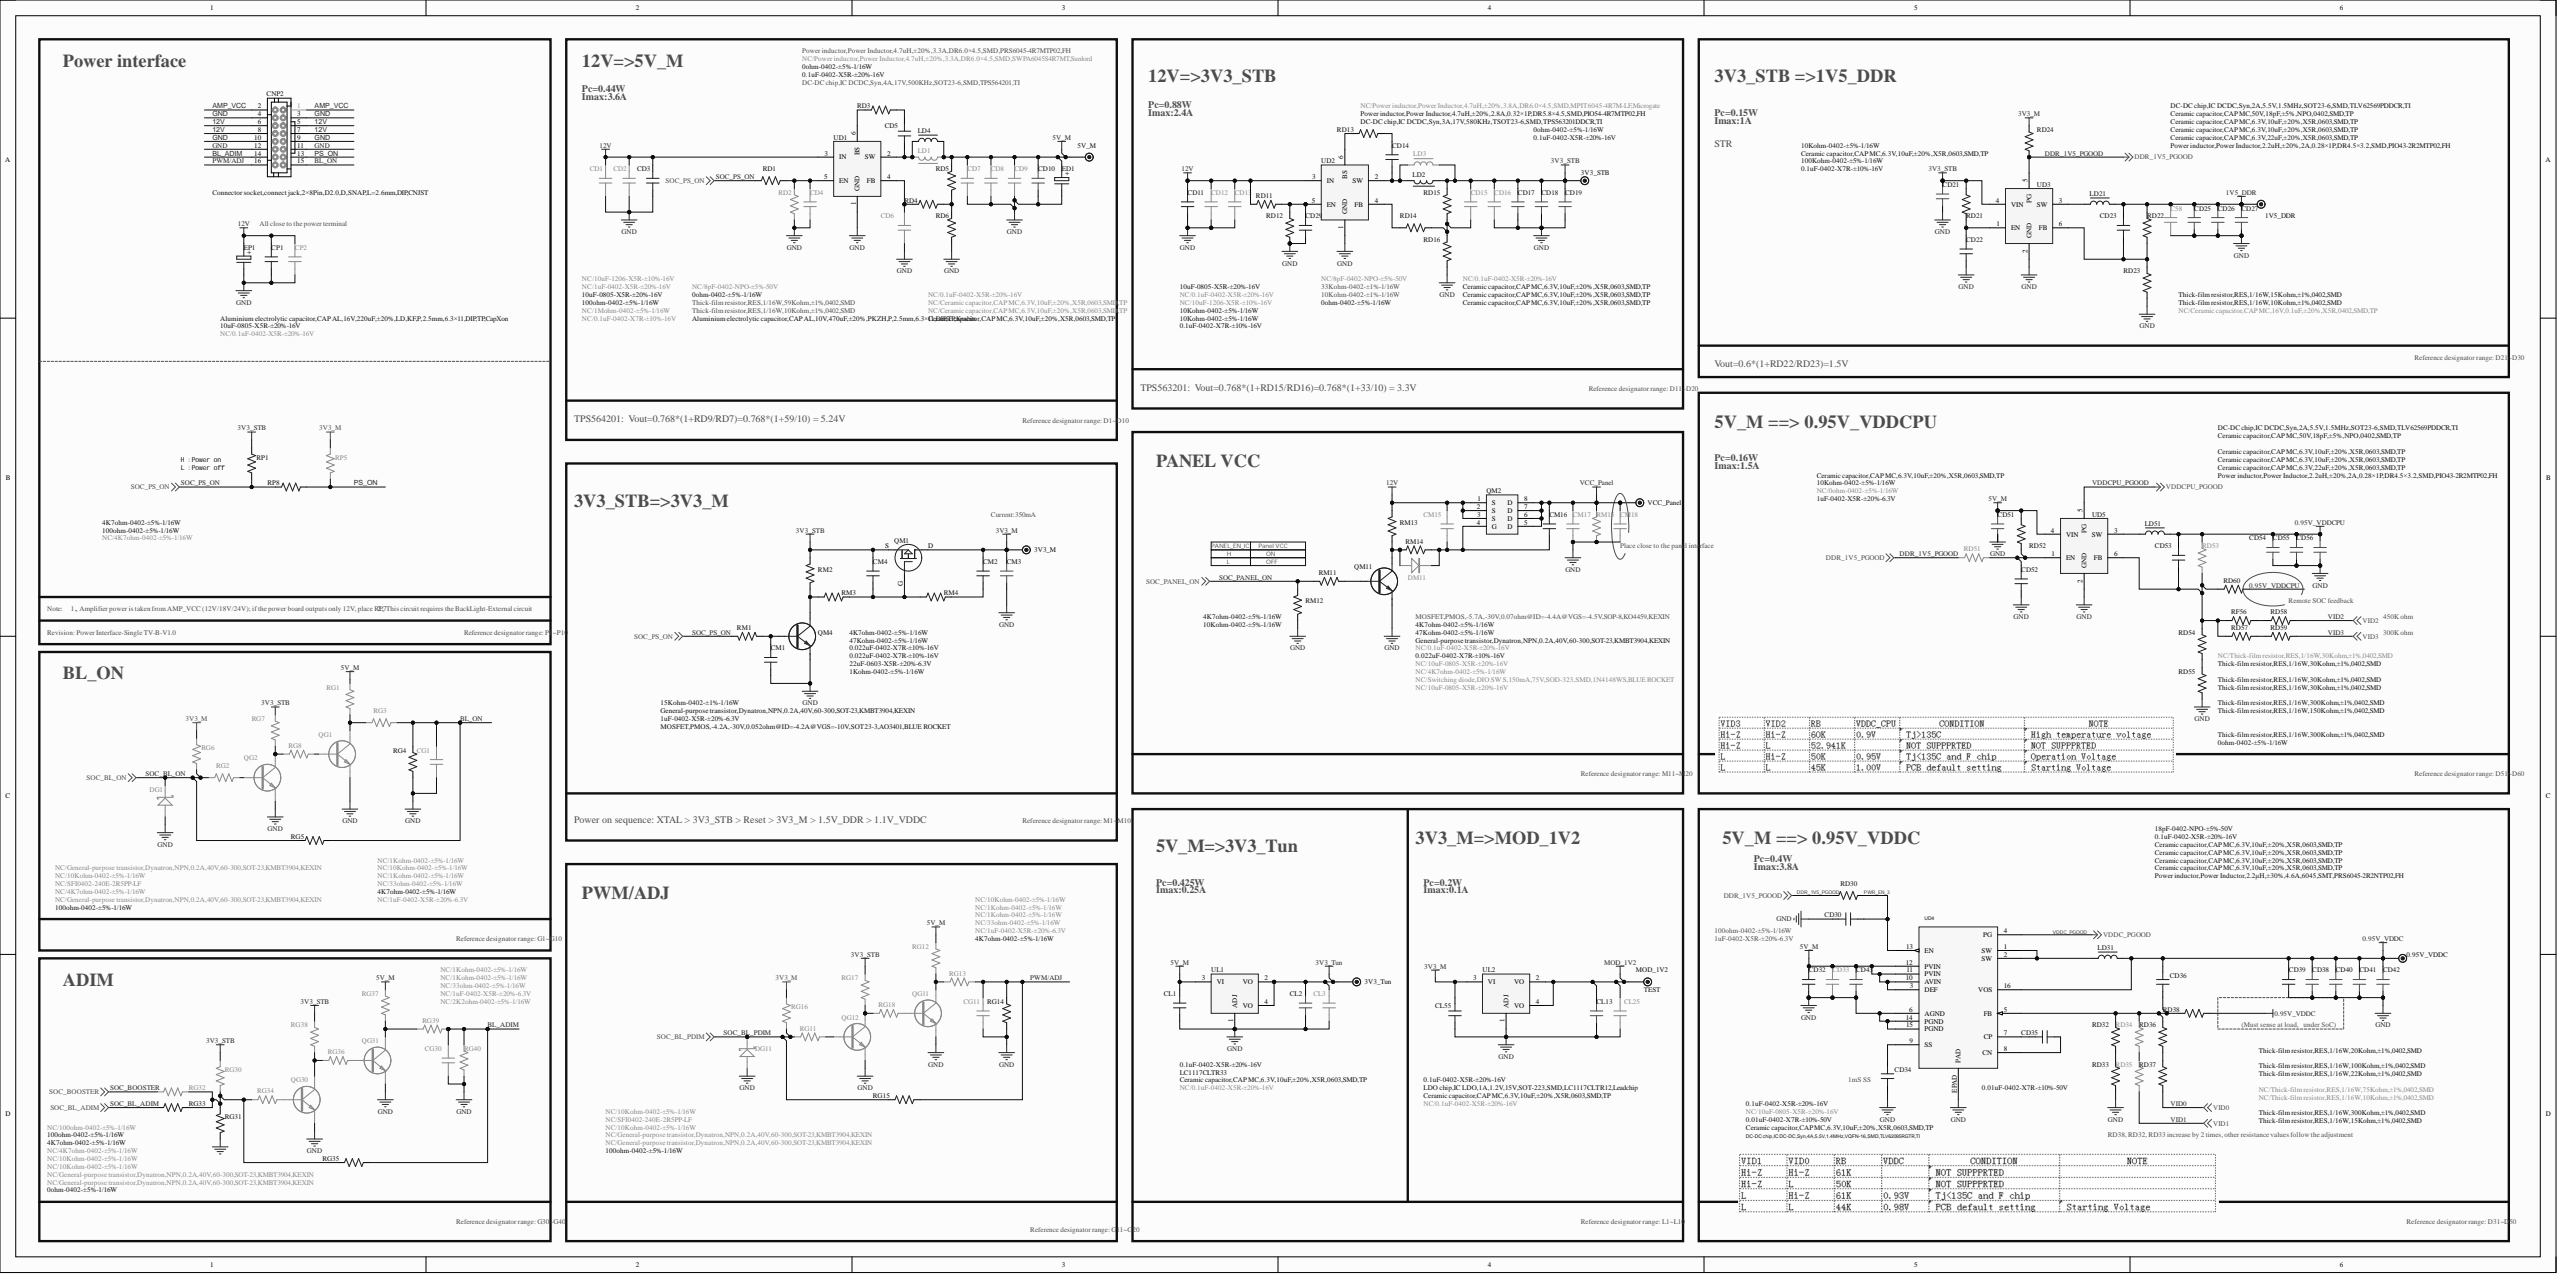Circuit board | Altium Designer | 1029 parts | 642 nets | one sheet of the schematic
Parts on this sheet (reference | value | footprint):
0.95V_VDDC | TEST | TP
1V5_DDR | TEST | TP
3V3_STB | TEST | TP
3V3_Tun | TEST | TP
5V_M | TEST | TP
C58 | NC/Ceramic capacitor,CAP MC,16V,0.1uF,±20%,X5R,0402,SMD,TP | C0402
CD1 | NC/10uF-1206-X5R-±10%-16V | C1206
CD2 | NC/1uF-0402-X5R-±20%-16V | C0402
CD3 | 10uF-0805-X5R-±20%-16V | C0805
CD4 | NC/0.1uF-0402-X7R-±10%-16V | C0402
CD5 | 0.1uF-0402-X5R-±20%-16V | C0402
CD6 | NC/8pF-0402-NPO-±5%-50V | C0402
CD7 | NC/0.1uF-0402-X5R-±20%-16V | C0402
CD8 | NC/Ceramic capacitor,CAP MC,6.3V,10uF,±20%,X5R,0603,SMD,TP | C0603
CD9 | NC/Ceramic capacitor,CAP MC,6.3V,10uF,±20%,X5R,0603,SMD,TP | C0603
CD10 | Ceramic capacitor,CAP MC,6.3V,10uF,±20%,X5R,0603,SMD,TP | C0603
CD11 | 10uF-0805-X5R-±20%-16V | C0805
CD12 | NC/0.1uF-0402-X5R-±20%-16V | C0402
CD13 | NC/10uF-1206-X5R-±10%-16V | C1206
CD14 | 0.1uF-0402-X5R-±20%-16V | C0402
CD15 | NC/8pF-0402-NPO-±5%-50V | C0402
CD16 | NC/0.1uF-0402-X5R-±20%-16V | C0402
CD17 | Ceramic capacitor,CAP MC,6.3V,10uF,±20%,X5R,0603,SMD,TP | C0603
CD18 | Ceramic capacitor,CAP MC,6.3V,10uF,±20%,X5R,0603,SMD,TP | C0603
CD19 | Ceramic capacitor,CAP MC,6.3V,10uF,±20%,X5R,0603,SMD,TP | C0603
CD21 | Ceramic capacitor,CAP MC,6.3V,10uF,±20%,X5R,0603,SMD,TP | C0603
CD22 | 0.1uF-0402-X7R-±10%-16V | C0402
CD23 | Ceramic capacitor,CAP MC,50V,18pF,±5%,NPO,0402,SMD,TP | C0402
CD25 | Ceramic capacitor,CAP MC,6.3V,10uF,±20%,X5R,0603,SMD,TP | C0603
CD26 | Ceramic capacitor,CAP MC,6.3V,10uF,±20%,X5R,0603,SMD,TP | C0603
CD27 | Ceramic capacitor,CAP MC,6.3V,22uF,±20%,X5R,0603,SMD,TP | C0603
CD29 | 0.1uF-0402-X7R-±10%-16V | C0402
CD30 | 1uF-0402-X5R-±20%-6.3V | C0402
CD32 | 0.1uF-0402-X5R-±20%-16V | C0402
CD33 | NC/10uF-0805-X5R-±20%-16V | C0805
CD34 | 0.01uF-0402-X7R-±10%-50V | C0402
CD35 | 0.01uF-0402-X7R-±10%-50V | C0402
CD36 | 18pF-0402-NPO-±5%-50V | C0402
CD38 | Ceramic capacitor,CAP MC,6.3V,10uF,±20%,X5R,0603,SMD,TP | C0603
CD39 | 0.1uF-0402-X5R-±20%-16V | C0402
CD40 | Ceramic capacitor,CAP MC,6.3V,10uF,±20%,X5R,0603,SMD,TP | C0603
CD41 | Ceramic capacitor,CAP MC,6.3V,10uF,±20%,X5R,0603,SMD,TP | C0603
CD42 | Ceramic capacitor,CAP MC,6.3V,10uF,±20%,X5R,0603,SMD,TP | C0603
CD43 | Ceramic capacitor,CAP MC,6.3V,10uF,±20%,X5R,0603,SMD,TP | C0603
CD51 | Ceramic capacitor,CAP MC,6.3V,10uF,±20%,X5R,0603,SMD,TP | C0603
CD52 | 1uF-0402-X5R-±20%-6.3V | C0402
CD53 | Ceramic capacitor,CAP MC,50V,18pF,±5%,NPO,0402,SMD,TP | C0402
CD54 | Ceramic capacitor,CAP MC,6.3V,10uF,±20%,X5R,0603,SMD,TP | C0603
CD55 | Ceramic capacitor,CAP MC,6.3V,10uF,±20%,X5R,0603,SMD,TP | C0603
CD56 | Ceramic capacitor,CAP MC,6.3V,22uF,±20%,X5R,0603,SMD,TP | C0603
CG1 | NC/1uF-0402-X5R-±20%-6.3V | C0402
CG11 | NC/1uF-0402-X5R-±20%-6.3V | C0402
CG30 | NC/1uF-0402-X5R-±20%-6.3V | C0402
CL1 | 0.1uF-0402-X5R-±20%-16V | C0402
CL2 | Ceramic capacitor,CAP MC,6.3V,10uF,±20%,X5R,0603,SMD,TP | C0603
CL3 | NC/0.1uF-0402-X5R-±20%-16V | C0402
CL13 | Ceramic capacitor,CAP MC,6.3V,10uF,±20%,X5R,0603,SMD,TP | C0603
CL25 | NC/0.1uF-0402-X5R-±20%-16V | C0402
CL55 | 0.1uF-0402-X5R-±20%-16V | C0402
CM1 | 1uF-0402-X5R-±20%-6.3V | C0402
CM2 | 0.022uF-0402-X7R-±10%-16V | C0402
CM3 | 22uF-0603-X5R-±20%-6.3V | C0603
CM4 | 0.022uF-0402-X7R-±10%-16V | C0402
CM15 | NC/0.1uF-0402-X5R-±20%-16V | C0402
CM16 | 0.022uF-0402-X7R-±10%-16V | C0402
CM17 | NC/10uF-0805-X5R-±20%-16V | C0805
CM18 | NC/10uF-0805-X5R-±20%-16V | C0805
CNP2 | Connector socket,connect jack,2×8Pin,D2.0,D,SNAP,L=2.6mm,DIP,CNJST | SIP2*8/2.0D-5
CP1 | 10uF-0805-X5R-±20%-16V | C0805
CP2 | NC/0.1uF-0402-X5R-±20%-16V | C0402
DG1 | NC/SFI0402-240E-2R5PP-LF | DIODE-S0402
DG11 | NC/SFI0402-240E-2R5PP-LF | DIODE-S0402
DM11 | NC/Switching diode,DIO SW S,150mA,75V,SOD-323,SMD,1N4148WS,BLUE ROCKET | DIODE-S-12
LD1 | NC/Power inductor,Power Inductor,4.7uH,±20%,3.3A,DR6.0×4.5,SMD,SWPA6045S4R7MT,Sunlord | L(6.0*4.5)-S
LD2 | Power inductor,Power Inductor,4.7uH,±20%,2.8A,0.32×1P,DR5.8×4.5,SMD,PIO54-4R7MTP02,FH | L(5.8*4.5)-S
LD3 | NC/Power inductor,Power Inductor,4.7uH,±20%,3.8A,DR6.0×4.5,SMD,MPIT6045-4R7M-LF,Microgate | L(6.0*4.5)-S
LD4 | Power inductor,Power Inductor,4.7uH,±20%,3.3A,DR6.0×4.5,SMD,PRS6045-4R7MTP02,FH | L(6.0*4.5)-S
LD21 | Power inductor,Power Inductor,2.2uH,±20%,2A,0.28×1P,DR4.5×3.2,SMD,PIO43-2R2MTP02,FH | L(4.5*3.5)-S
LD31 | Power inductor,Power Inductor,2.2µH,±30%,4.6A,6045,SMT,PRS6045-2R2NTP02,FH | L(6.0*4.5)-S
LD51 | Power inductor,Power Inductor,2.2uH,±20%,2A,0.28×1P,DR4.5×3.2,SMD,PIO43-2R2MTP02,FH | L(4.5*3.5)-S
MOD_1V2 | TEST | TP
QG1 | NC/General-purpose transistor,Dynatron,NPN,0.2A,40V,60-300,SOT-23,KMBT3904,KEXIN | SOT-23
QG2 | NC/General-purpose transistor,Dynatron,NPN,0.2A,40V,60-300,SOT-23,KMBT3904,KEXIN | SOT-23
QG11 | NC/General-purpose transistor,Dynatron,NPN,0.2A,40V,60-300,SOT-23,KMBT3904,KEXIN | SOT-23
QG12 | NC/General-purpose transistor,Dynatron,NPN,0.2A,40V,60-300,SOT-23,KMBT3904,KEXIN | SOT-23
QG30 | NC/General-purpose transistor,Dynatron,NPN,0.2A,40V,60-300,SOT-23,KMBT3904,KEXIN | SOT-23
QG31 | NC/General-purpose transistor,Dynatron,NPN,0.2A,40V,60-300,SOT-23,KMBT3904,KEXIN | SOT-23
QM4 | General-purpose transistor,Dynatron,NPN,0.2A,40V,60-300,SOT-23,KMBT3904,KEXIN | SOT-23
QM11 | General-purpose transistor,Dynatron,NPN,0.2A,40V,60-300,SOT-23,KMBT3904,KEXIN | SOT-23
RD1 | 100ohm-0402-±5%-1/16W | R0402
RD2 | NC/1Mohm-0402-±5%-1/16W | R0402
RD3 | 0ohm-0402-±5%-1/16W | R0402
RD4 | 0ohm-0402-±5%-1/16W | R0402
RD5 | Thick-film resistor,RES,1/16W,59Kohm,±1%,0402,SMD | R0402
RD6 | Thick-film resistor,RES,1/16W,10Kohm,±1%,0402,SMD | R0402
RD11 | 10Kohm-0402-±5%-1/16W | R0402
RD12 | 10Kohm-0402-±5%-1/16W | R0402
RD13 | 0ohm-0402-±5%-1/16W | R0402
RD14 | 0ohm-0402-±5%-1/16W | R0402
RD15 | 33Kohm-0402-±1%-1/16W | R0402
RD16 | 10Kohm-0402-±1%-1/16W | R0402
RD21 | 100Kohm-0402-±5%-1/16W | R0402
RD22 | Thick-film resistor,RES,1/16W,15Kohm,±1%,0402,SMD | R0402
RD23 | Thick-film resistor,RES,1/16W,10Kohm,±1%,0402,SMD | R0402
RD24 | 10Kohm-0402-±5%-1/16W | R0402
RD30 | 100ohm-0402-±5%-1/16W | R0402
RD32 | Thick-film resistor,RES,1/16W,100Kohm,±1%,0402,SMD | R0402
RD33 | Thick-film resistor,RES,1/16W,22Kohm,±1%,0402,SMD | R0402
RD34 | NC/Thick-film resistor,RES,1/16W,75Kohm,±1%,0402,SMD | R0402
RD35 | NC/Thick-film resistor,RES,1/16W,10Kohm,±1%,0402,SMD | R0402
RD36 | Thick-film resistor,RES,1/16W,300Kohm,±1%,0402,SMD | R0402
RD37 | Thick-film resistor,RES,1/16W,15Kohm,±1%,0402,SMD | R0402
RD38 | Thick-film resistor,RES,1/16W,20Kohm,±1%,0402,SMD | R0402
RD51 | NC/0ohm-0402-±5%-1/16W | R0402
RD52 | 10Kohm-0402-±5%-1/16W | R0402
RD53 | NC/Thick-film resistor,RES,1/16W,30Kohm,±1%,0402,SMD | R0402
RD54 | Thick-film resistor,RES,1/16W,30Kohm,±1%,0402,SMD | R0402
RD55 | Thick-film resistor,RES,1/16W,30Kohm,±1%,0402,SMD | R0402
RD57 | Thick-film resistor,RES,1/16W,300Kohm,±1%,0402,SMD | R0402
RD58 | Thick-film resistor,RES,1/16W,150Kohm,±1%,0402,SMD | R0402
RD59 | 0ohm-0402-±5%-1/16W | R0402
RD60 | Thick-film resistor,RES,1/16W,30Kohm,±1%,0402,SMD | R0402
RF56 | Thick-film resistor,RES,1/16W,300Kohm,±1%,0402,SMD | R0402
RG1 | NC/1Kohm-0402-±5%-1/16W | R0402
RG2 | NC/4K7ohm-0402-±5%-1/16W | R0402
RG3 | NC/33ohm-0402-±5%-1/16W | R0402
RG4 | 4K7ohm-0402-±5%-1/16W | R0402
RG5 | 100ohm-0402-±5%-1/16W | R0402
RG6 | NC/10Kohm-0402-±5%-1/16W | R0402
RG7 | NC/1Kohm-0402-±5%-1/16W | R0402
RG8 | NC/10Kohm-0402-±5%-1/16W | R0402
RG11 | NC/10Kohm-0402-±5%-1/16W | R0402
RG12 | NC/1Kohm-0402-±5%-1/16W | R0402
RG13 | NC/33ohm-0402-±5%-1/16W | R0402
RG14 | 4K7ohm-0402-±5%-1/16W | R0402
RG15 | 100ohm-0402-±5%-1/16W | R0402
RG16 | NC/10Kohm-0402-±5%-1/16W | R0402
RG17 | NC/1Kohm-0402-±5%-1/16W | R0402
RG18 | NC/10Kohm-0402-±5%-1/16W | R0402
RG30 | NC/4K7ohm-0402-±5%-1/16W | R0402
RG31 | 4K7ohm-0402-±5%-1/16W | R0402
RG32 | NC/100ohm-0402-±5%-1/16W | R0402
RG33 | 100ohm-0402-±5%-1/16W | R0402
RG34 | NC/10Kohm-0402-±5%-1/16W | R0402
RG35 | 0ohm-0402-±5%-1/16W | R0402
RG36 | NC/10Kohm-0402-±5%-1/16W | R0402
RG37 | NC/1Kohm-0402-±5%-1/16W | R0402
RG38 | NC/1Kohm-0402-±5%-1/16W | R0402
RG39 | NC/33ohm-0402-±5%-1/16W | R0402
RG40 | NC/2K2ohm-0402-±5%-1/16W | R0402
RM1 | 15Kohm-0402-±1%-1/16W | R0402
RM2 | 4K7ohm-0402-±5%-1/16W | R0402
RM3 | 47Kohm-0402-±5%-1/16W | R0402
RM4 | 1Kohm-0402-±5%-1/16W | R0402
RM11 | 4K7ohm-0402-±5%-1/16W | R0402
RM12 | 10Kohm-0402-±5%-1/16W | R0402
RM13 | 4K7ohm-0402-±5%-1/16W | R0402
RM14 | 47Kohm-0402-±5%-1/16W | R0402
RM15 | NC/4K7ohm-0402-±5%-1/16W | R0402
RP1 | 4K7ohm-0402-±5%-1/16W | R0402
RP5 | NC/4K7ohm-0402-±5%-1/16W | R0402
RP8 | 100ohm-0402-±5%-1/16W | R0402
UD1 | DC-DC chip,IC DCDC,Syn,4A,17V,500KHz,SOT23-6,SMD,TPS564201,TI | SOP6/0.95
UD2 | DC-DC chip,IC DCDC,Syn,3A,17V,580KHz,TSOT23-6,SMD,TPS563201DDCR,TI | SOP6/0.95
UD3 | DC-DC chip,IC DCDC,Syn,2A,5.5V,1.5MHz,SOT23-6,SMD,TLV62569PDDCR,TI | SOT-23-6
UD4 | DC-DC chip,IC DC-DC,Syn,4A,5.5V,1.4MHz,VQFN-16,SMD,TLV62095RGTR,TI | QFN16/0.5-4
UD5 | DC-DC chip,IC DCDC,Syn,2A,5.5V,1.5MHz,SOT23-6,SMD,TLV62569PDDCR,TI | SOT-23-6
UL1 | LC1117CLTR33 | SOT-223
UL2 | LDO chip,IC LDO,1A,1.2V,15V,SOT-223,SMD,LC1117CLTR12,Leadchip | SOT-223
VCC_Panel | TEST | TP
Nets of these parts (net: part-pin ...):
VID3: RD59-1
VID2: RD58-1
VID1: RD35-1
VID0: RD37-1
VDDCPU_PGOOD: UD5-5
VDDC_PGOOD: UD4-4
VCC_Panel: CM16-2 CM17-1 CM18-1 RM15-1 VCC_Panel-1
SOC_PS_ON: RD1-1 RM1-1 RP1-1 RP8-2
SOC_PANEL_ON: RM11-1 RM12-2
SOC_BOOSTER: RG32-1
SOC_BL_PDIM: DG11-K RG11-2 RG15-2 RG16-1
SOC_BL_ON: DG1-K RG2-2 RG5-2 RG6-1
SOC_BL_ADIM: RG33-1
PWR_EN_3: CD30-2 RD30-2 UD4-13
PWM/ADJ: CG11-2 CNP2-16 RG13-2 RG14-2 RG15-1
PS_ON: CNP2-13 RP5-1 RP8-1
NetRG30_1: RG30-1 RG31-2 RG32-2 RG33-2 RG34-2 RG35-2
NetRD58_2: RD58-2 RF56-1
NetRD57_1: RD57-1 RD59-2
NetRD54_1: RD54-1 RD55-2
NetRD36_2: RD36-2 RD37-2
NetRD34_2: RD34-2 RD35-2
NetRD32_2: RD32-2 RD33-2
NetRD14_1: RD14-1 UD2-4
NetRD13_1: RD13-1 UD2-6
NetRD4_2: RD4-2 RD5-2 RD6-2
NetRD3_1: RD3-1 UD1-6
NetQM11_B: QM11-B RM11-2
NetQM4_C: QM4-C RM2-2 RM3-1
NetQG31_C: QG31-C RG37-1 RG39-1
NetQG31_B: QG31-B RG36-1
NetQG30_C: QG30-C RG36-2 RG38-1
NetQG30_B: QG30-B RG34-1
NetQG12_C: QG12-C RG17-1 RG18-2
NetQG12_B: QG12-B RG11-1
NetQG11_C: QG11-C RG12-1 RG13-1
NetQG11_B: QG11-B RG18-1
NetQG2_C: QG2-C RG7-1 RG8-2
NetQG2_B: QG2-B RG2-1
NetQG1_C: QG1-C RG1-1 RG3-2
NetQG1_B: QG1-B RG8-1
NetLD51_1: LD51-1 UD5-3
NetLD31_1: LD31-1 UD4-1 UD4-2
NetLD21_1: LD21-1 UD3-3
NetDM11_A: DM11-A QM11-C RM13-2 RM14-1
NetCM15_1: CM15-1 CM16-1 DM11-K RM14-2
NetCM4_1: CM4-1 RM3-2 RM4-1
NetCM2_1: CM2-1 RM4-2
NetCM1_2: CM1-2 QM4-B RM1-2
NetCD53_1: CD53-1 RD53-1 RD54-2 RD57-2 RD60-2 RF56-2 UD5-6
NetCD52_1: CD52-1 RD51-1 RD52-1 UD5-1
NetCD36_1: CD36-1 RD32-1 RD34-1 RD36-1 RD38-1 UD4-5
NetCD35_2: CD35-2 UD4-7
NetCD35_1: CD35-1 UD4-8
NetCD34_2: CD34-2 UD4-9
NetCD29_1: CD29-1 RD11-2 RD12-2 UD2-5
NetCD23_1: CD23-1 RD22-1 RD23-2 UD3-6
NetCD22_1: CD22-1 RD21-1 UD3-1
NetCD15_1: CD15-1 RD14-2 RD15-2 RD16-2
NetCD14_2: CD14-2 RD13-2
NetCD14_1: CD14-1 LD2-2 LD3-1 UD2-2
NetCD6_2: CD6-2 RD4-1 UD1-4
NetCD5_2: CD5-2 LD1-1 LD4-1 UD1-2
NetCD5_1: CD5-1 RD3-2
NetCD4_1: CD4-1 RD1-2 RD2-2 UD1-5
MOD_1V2: CL13-2 CL25-2 MOD_1V2-1 UL2-2 UL2-4
GND: C58-1 CD1-1 CD2-1 CD3-2 CD4-2 CD6-1 CD7-1 CD8-1 CD9-1 CD10-1 CD11-2 CD12-1 CD13-1 CD16-1 CD17-1 CD18-1 CD19-1 CD21-1 CD22-2 CD25-1 CD26-1 CD27-1 CD29-2 CD30-1 CD32-1 CD33-2 CD34-1 CD38-1 CD39-1 CD40-1 CD41-1 CD42-1 CD43-1 CD51-1 CD52-2 CD54-1 CD55-1 CD56-1 CG1-1 CG11-1 CG30-1 CL1-2 CL2-1 CL3-2 CL13-1 CL25-1 CL55-1 CM1-1 CM3-1 CM17-2 CM18-2 CNP2-3 CNP2-4 CNP2-9 CNP2-10 CNP2-11 CNP2-12 CP1-1 CP2-1 DG1-A DG11-A QG1-E QG2-E QG11-E QG12-E QG30-E QG31-E QM4-E QM11-E RD2-1 RD6-1 RD12-1 RD16-1 RD23-1 RD33-1 RD55-1 RG4-1 RG14-1 RG31-1 RG40-1 RM12-1 RM15-2 UD1-1 UD2-1 UD3-2 UD4-6 UD4-14 UD4-15 UD4-EPAD UD5-2 UL1-1 UL2-1
DDR_1V5_PGOOD: RD24-1 RD30-1 RD51-2 UD3-5
BL_ON: CG1-2 CNP2-15 RG3-1 RG4-2 RG5-1
BL_ADIM: CG30-2 CNP2-14 RG35-1 RG39-2 RG40-2
AMP_VCC: CNP2-1 CNP2-2
12V: CD1-2 CD2-2 CD3-1 CD11-1 CD12-2 CD13-2 CM15-2 CNP2-5 CNP2-6 CNP2-7 CNP2-8 CP1-2 CP2-2 RD11-1 RM13-1 UD1-3 UD2-3
5V_M: 5V_M-1 CD7-2 CD8-2 CD9-2 CD10-2 CD32-2 CD33-1 CD43-2 CD51-2 CL1-1 LD1-2 LD4-2 RD5-1 RD52-2 RG1-2 RG12-2 RG37-2 UD4-3 UD4-10 UD4-11 UD4-12 UD5-4 UL1-3
3V3_Tun: 3V3_Tun-1 CL2-2 CL3-1 UL1-2 UL1-4
3V3_STB: 3V3_STB-1 CD15-2 CD16-2 CD17-2 CD18-2 CD19-2 CD21-2 CM4-2 LD2-1 LD3-2 RD15-1 RD21-2 RG7-2 RG17-2 RG30-2 RG38-2 RM2-1 RP1-2 UD3-4
3V3_M: CL55-2 CM2-2 CM3-2 RD24-2 RG6-2 RG16-2 RP5-2 UL2-3
1V5_DDR: 1V5_DDR-1 C58-2 CD23-2 CD25-2 CD26-2 CD27-2 LD21-2 RD22-2
0.95V_VDDCPU: CD53-2 CD54-2 CD55-2 CD56-2 LD51-2 RD53-2 RD60-1
0.95V_VDDC: 0.95V_VDDC-1 CD36-2 CD38-2 CD39-2 CD40-2 CD41-2 CD42-2 LD31-2 RD38-2 UD4-16